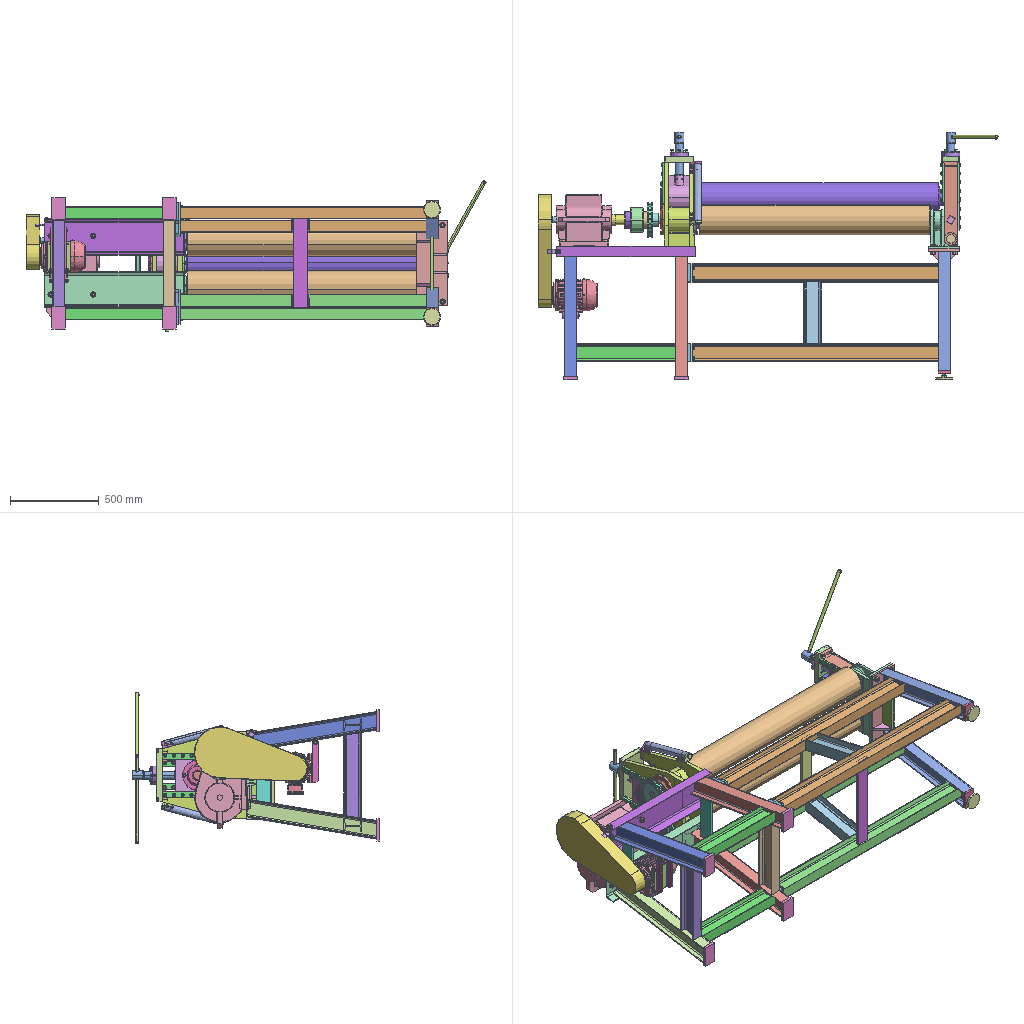Assembly | SolidWorks | 110 different items | 393 placed | box 2588 x 1390 x 851 mm
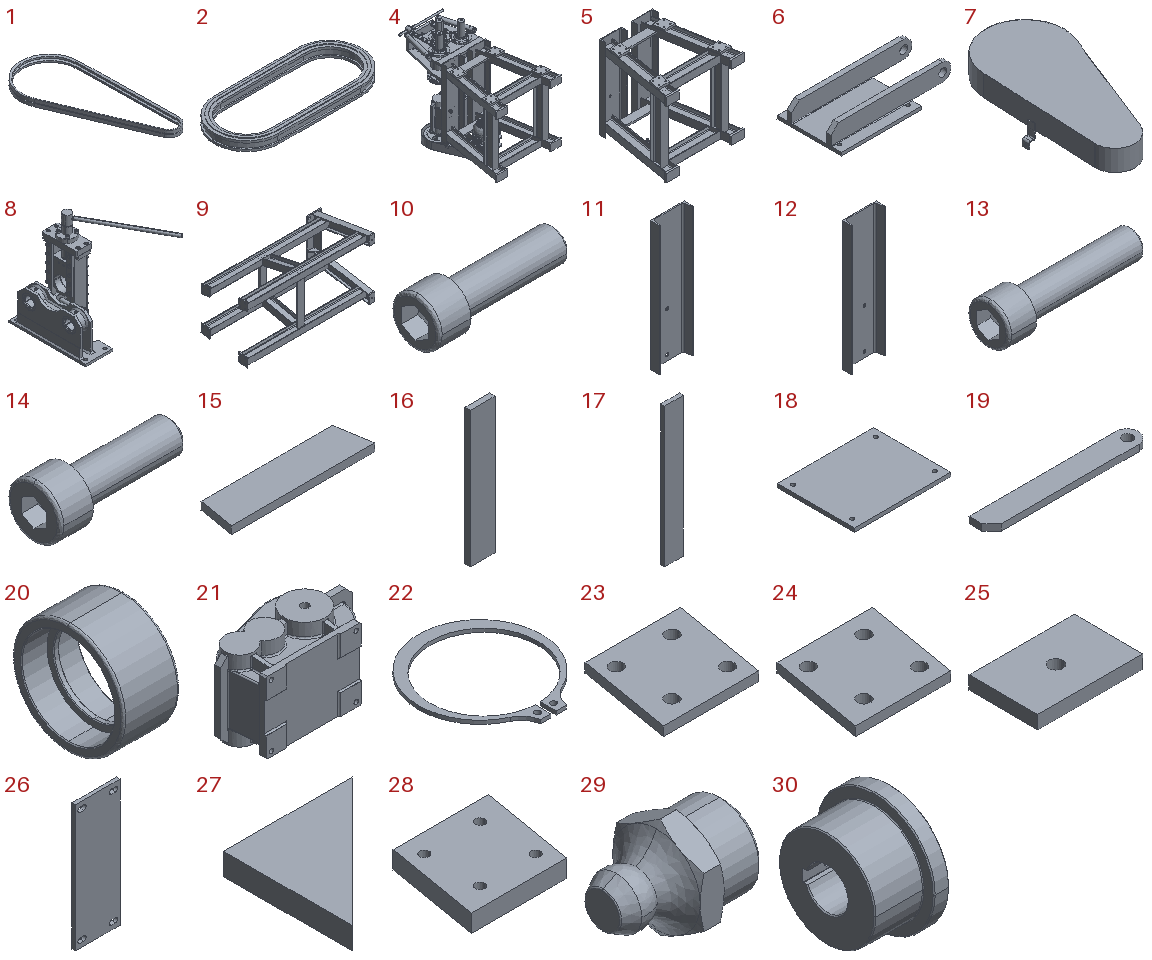Parts list (item | name | quantity | parent item | size | volume | features):
1 | (subassembly) | x1 | in 4 | 255.391 x 589.134 x 28.445 mm | 211928 mm3 | -
2 | (subassembly) | x1 | in 4 | 444.526 x 194.526 x 33.528 mm | 618540 mm3 | -
3 | (subassembly) | x1 | - | - | - | -
4 | (subassembly) | x1 | - | - | 68898357 mm3 | -
5 | (subassembly) | x1 | in 4 | 738.903 x 747.997 x 780 mm | 12463508 mm3 | -
6 | (subassembly) | x1 | in 4 | 244.844 x 131 x 41.4 mm | 299853 mm3 | -
7 | (subassembly) | x1 | in 4 | 319.788 x 636.5 x 127.78 mm | 416988 mm3 | -
8 | (subassembly) | x1 | - | 388.966 x 706.727 x 655.972 mm | 9412553 mm3 | -
9 | (subassembly) | x1 | - | 1510 x 699 x 705.243 mm | 14014214 mm3 | -
10 | - | x4 | in 8 | 52 x 18 x 18 mm | 6907 mm3 | features BaseBody 1
11 | - | x1 | in 5 | 203.2 x 57.4 x 780 mm | 1609191 mm3 | features BaseBody 1
12 | - | x1 | in 5 | 203.2 x 57.4 x 780 mm | 1609191 mm3 | features BaseBody 1
13 | - | x12 | in 4, 8 | 62 x 18 x 18 mm | 8038 mm3 | features BaseBody 1
14 | - | x8 | in 4 | 33 x 13 x 13 mm | 2157 mm3 | features BaseBody 1
15 | - | x1 | in 9 | 300.429 x 76.2 x 16 mm | 350736 mm3 | features BaseBody 1
16 | - | x1 | in 9 | 76 x 16 x 413.5 mm | 502816 mm3 | features BaseBody 1
17 | - | x1 | in 9 | 76 x 16 x 563.5 mm | 685216 mm3 | features BaseBody 1
18 | - | x1 | in 6 | 164 x 131 x 6.4 mm | 136609 mm3 | features BaseBody 1
19 | - | x2 | in 6 | 244.844 x 35 x 10 mm | 81253 mm3 | features BaseBody 1
20 | - | x1 | in 4 | 70 x 138 x 138 mm | 337126 mm3 | features BaseBody 1
21 | - | x1 | in 4 | 510 x 292.394 x 310 mm | 26978776 mm3 | features BaseBody 1
22 | - | x3 | in 4 | 54 x 59.172 x 1.6 mm | 946.092 mm3 | features BaseBody 1
23 | - | x2 | in 9 | 120.015 x 101.6 x 10 mm | 98503 mm3 | features BaseBody 1
24 | - | x2 | in 9 | 120.015 x 101.6 x 10 mm | 98503 mm3 | features BaseBody 1
25 | - | x2 | in 9 | 103 x 67.6 x 13 mm | 88562 mm3 | features BaseBody 1
26 | - | x1 | in 9 | 170 x 13 x 480 mm | 1034464 mm3 | features BaseBody 1
27 | - | x4 | in 9 | 76 x 76 x 13 mm | 37544 mm3 | features BaseBody 1
28 | - | x4 | in 5 | 120.015 x 101.6 x 19 mm | 192760 mm3 | features BaseBody 1
29 | - | x3 | in 8 | 16 x 11 x 12.702 mm | 986.989 mm3 | features BaseBody 1
30 | - | x1 | in 4 | 65 x 115 x 115 mm | 415156 mm3 | features BaseBody 1
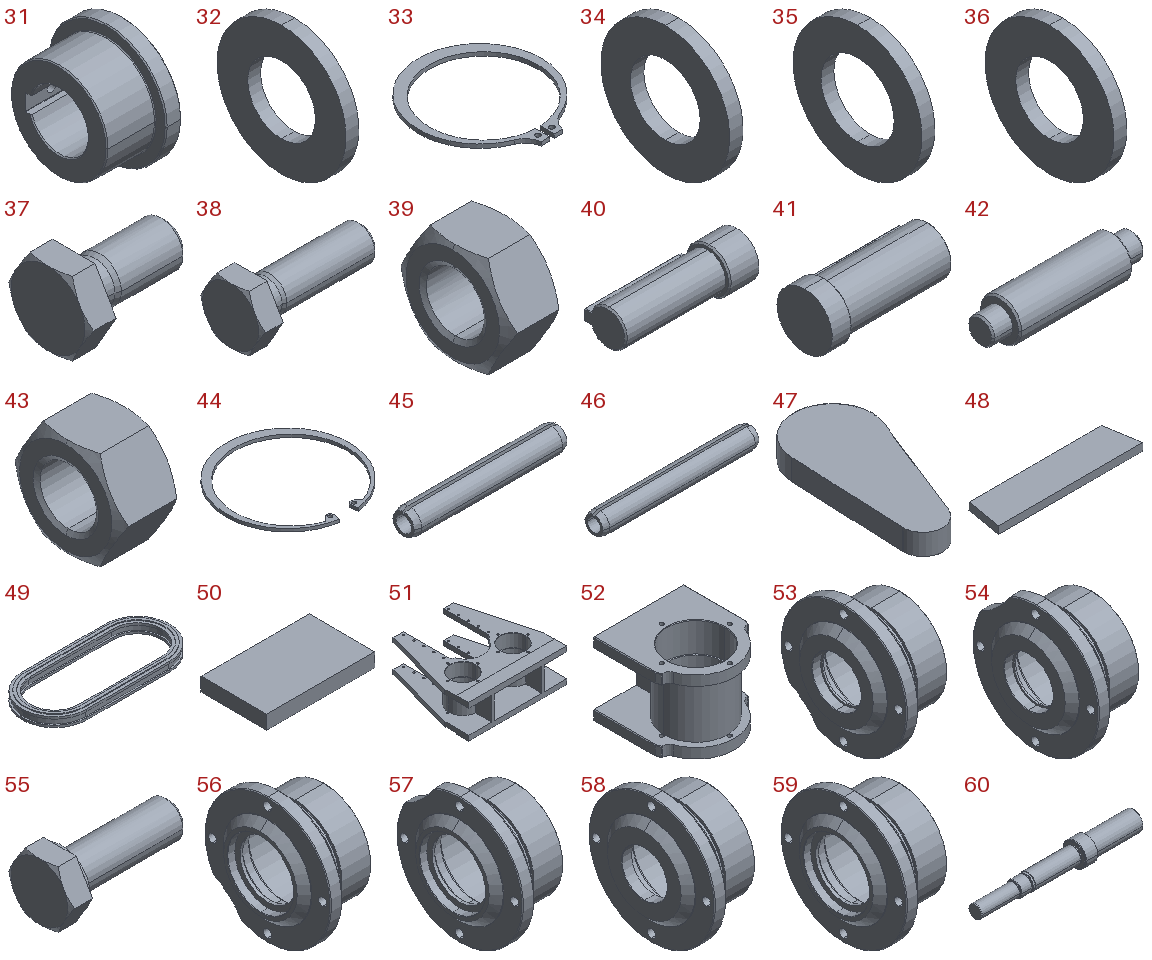31 | - | x1 | in 4 | 65 x 115 x 115 mm | 335130 mm3 | features BaseBody 1
32 | - | x70 | in 4, 8 | 2 x 20 x 20 mm | 455.138 mm3 | features BaseBody 1
33 | - | x1 | - | 64.433 x 69.873 x 2 mm | 1579 mm3 | features BaseBody 1
34 | - | x16 | - | 2.5 x 24 x 24 mm | 799.143 mm3 | features BaseBody 1
35 | - | x16 | in 4 | 3 x 30 x 30 mm | 1440 mm3 | features BaseBody 1
36 | - | x4 | in 4 | 1.6 x 16 x 16 mm | 233.031 mm3 | features BaseBody 1
37 | - | x2 | in 4 | 16 x 11.547 x 10 mm | 654.588 mm3 | features BaseBody 1
38 | - | x4 | in 4 | 30.3 x 15.011 x 13 mm | 1969 mm3 | features BaseBody 1
39 | - | x4 | in 4 | 13 x 27.713 x 24 mm | 4387 mm3 | features BaseBody 1
40 | - | x1 | in 4 | 93 x 33 x 32 mm | 57387 mm3 | features BaseBody 1
41 | - | x1 | in 4 | 145 x 66.5 x 65 mm | 388822 mm3 | features BaseBody 1
42 | - | x1 | in 5 | 94 x 25.4 x 25.4 mm | 40077 mm3 | features BaseBody 1
43 | - | x4 | - | 14.8 x 27.713 x 24 mm | 5033 mm3 | features BaseBody 1
44 | - | x6 | in 4 | 116.7 x 115.986 x 2.8 mm | 5057 mm3 | features BaseBody 1
45 | - | x2 | in 4 | 50 x 8 x 7.968 mm | 1446 mm3 | features BaseBody 1
46 | - | x2 | in 8 | 60 x 8 x 7.968 mm | 1740 mm3 | features BaseBody 1
47 | - | x1 | in 7 | 306.5 x 636.5 x 76.6 mm | 401718 mm3 | features BaseBody 1
48 | - | x2 | in 5 | 310.603 x 76.2 x 16 mm | 363141 mm3 | features BaseBody 1
49 | - | x1 | in 2 | 444.526 x 194.526 x 33.528 mm | 618540 mm3 | features BaseBody 1
50 | - | x4 | in 5 | 125 x 76.2 x 16 mm | 152400 mm3 | features BaseBody 1
51 | - | x1 | in 4 | 490 x 474 x 167.3 mm | 6268436 mm3 | features BaseBody 1
52 | - | x1 | in 4 | 200 x 210 x 160.5 mm | 1529038 mm3 | features BaseBody 1
53 | - | x1 | in 4 | 86.84 x 172 x 172 mm | 547122 mm3 | features BaseBody 1
54 | - | x1 | in 4 | 86.84 x 172 x 172 mm | 547344 mm3 | features BaseBody 1
55 | - | x26 | in 8 | 36.4 x 18.475 x 16 mm | 3746 mm3 | features BaseBody 1
56 | - | x1 | in 4 | 86.84 x 172 x 172 mm | 513296 mm3 | features BaseBody 1
57 | - | x1 | in 4 | 86.84 x 172 x 172 mm | 513518 mm3 | features BaseBody 1
58 | - | x1 | in 4 | 86.84 x 172 x 172 mm | 557963 mm3 | features BaseBody 1
59 | - | x1 | in 4 | 86.84 x 172 x 172 mm | 518697 mm3 | features BaseBody 1
60 | - | x1 | in 4 | 498.34 x 74 x 74 mm | 1078927 mm3 | features BaseBody 1
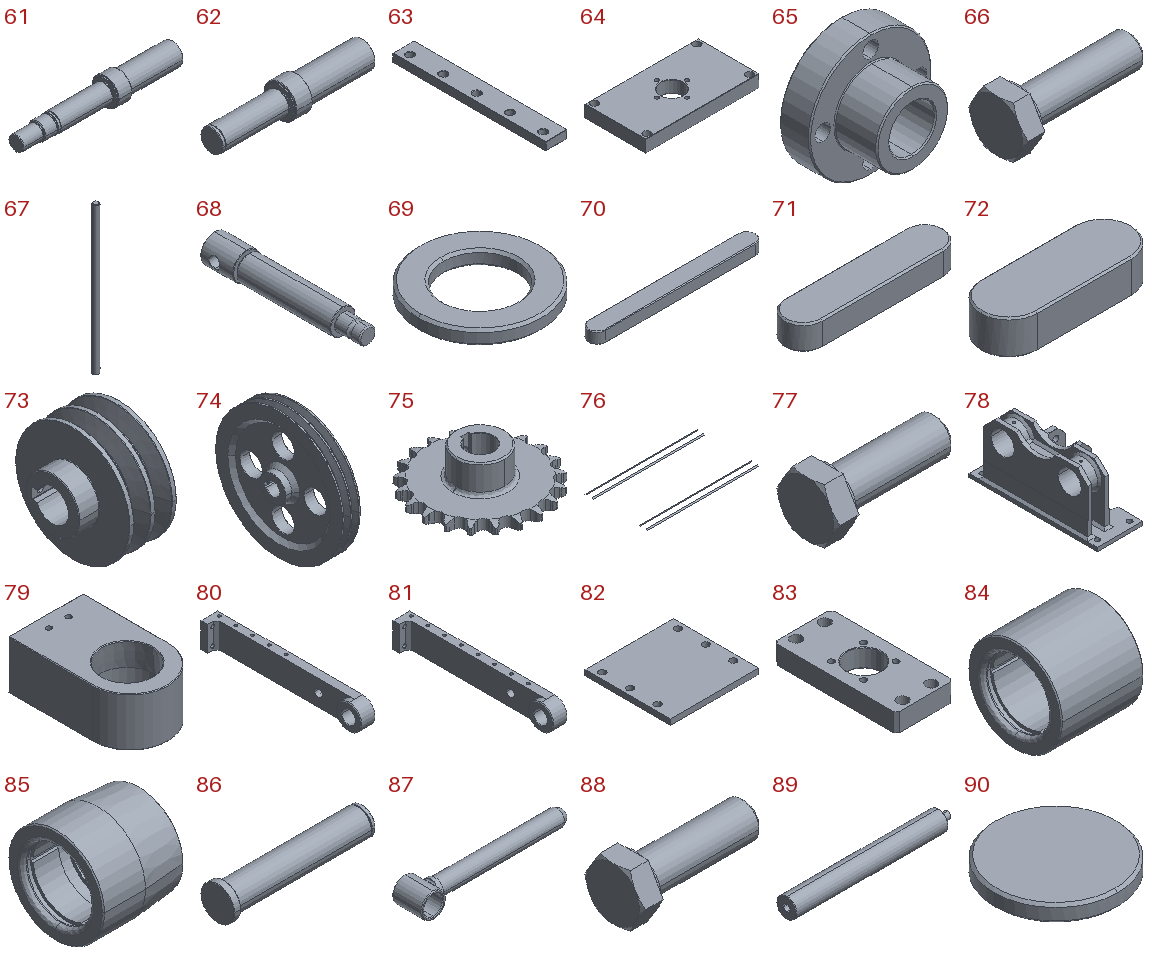61 | - | x1 | in 4 | 434.34 x 74 x 74 mm | 1002154 mm3 | features BaseBody 1
62 | - | x1 | in 4 | 341.34 x 74 x 74 mm | 870212 mm3 | features BaseBody 1
63 | - | x8 | in 4, 8 | 32 x 230 x 12 mm | 82466 mm3 | features BaseBody 1
64 | - | x1 | in 4 | 300 x 160.5 x 32 mm | 1414203 mm3 | features BaseBody 1
65 | - | x2 | in 4, 8 | 102 x 60 x 102 mm | 221417 mm3 | features BaseBody 1
66 | - | x44 | in 4 | 41.4 x 18.475 x 16 mm | 4138 mm3 | features BaseBody 1
67 | - | x2 | in 4, 8 | 23.05 x 19.05 x 500 mm | 142580 mm3 | features BaseBody 1
68 | - | x2 | in 4, 8 | 50.8 x 282 x 50.8 mm | 426019 mm3 | features BaseBody 1
69 | - | x2 | in 4, 8 | 50.8 x 50.8 x 6 mm | 7609 mm3 | features BaseBody 1
70 | - | x1 | in 4 | 116 x 12 x 8 mm | 10828 mm3 | features BaseBody 1
71 | - | x1 | in 4 | 51 x 12 x 8 mm | 4620 mm3 | features BaseBody 1
72 | - | x3 | in 4 | 48 x 18 x 11 mm | 8710 mm3 | features BaseBody 1
73 | - | x1 | in 4 | 50 x 85 x 85 mm | 143895 mm3 | features BaseBody 1
74 | - | x1 | in 4 | 47.331 x 248 x 248 mm | 1015220 mm3 | features BaseBody 1
75 | - | x2 | in 4 | 183.758 x 182.894 x 56.916 mm | 418597 mm3 | features BaseBody 1
76 | - | x1 | in 6 | 164 x 93 x 1.5 mm | 738 mm3 | features BaseBody 4
77 | - | x16 | - | 42.5 x 20.785 x 18 mm | 6020 mm3 | features BaseBody 1
78 | - | x1 | in 8 | 170 x 480 x 224 mm | 3738695 mm3 | features BaseBody 1
79 | - | x1 | in 8 | 115 x 187.5 x 75 mm | 1043413 mm3 | features BaseBody 1
80 | - | x1 | in 8 | 50 x 470 x 75 mm | 866067 mm3 | features BaseBody 1
81 | - | x1 | in 8 | 50 x 470 x 75 mm | 866067 mm3 | features BaseBody 1
82 | - | x1 | in 8 | 160 x 155 x 10 mm | 241214 mm3 | features BaseBody 1
83 | - | x1 | in 8 | 100 x 215 x 32 mm | 560281 mm3 | features BaseBody 1
84 | - | x2 | in 8 | 76 x 86 x 86 mm | 218570 mm3 | features BaseBody 1
85 | - | x1 | - | 75 x 85 x 85 mm | 185357 mm3 | features BaseBody 1
86 | - | x1 | in 8 | 215 x 50 x 50 mm | 276823 mm3 | features BaseBody 1
87 | - | x1 | in 8 | 211.2 x 40 x 33.4 mm | 81310 mm3 | features BaseBody 1
88 | - | x10 | in 4 | 60 x 27.713 x 24 mm | 14953 mm3 | features BaseBody 1
89 | - | x2 | - | 1379 x 168 x 168 mm | 11660432 mm3 | features BaseBody 1
90 | - | x2 | - | 95 x 95 x 13 mm | 90970 mm3 | features BaseBody 1
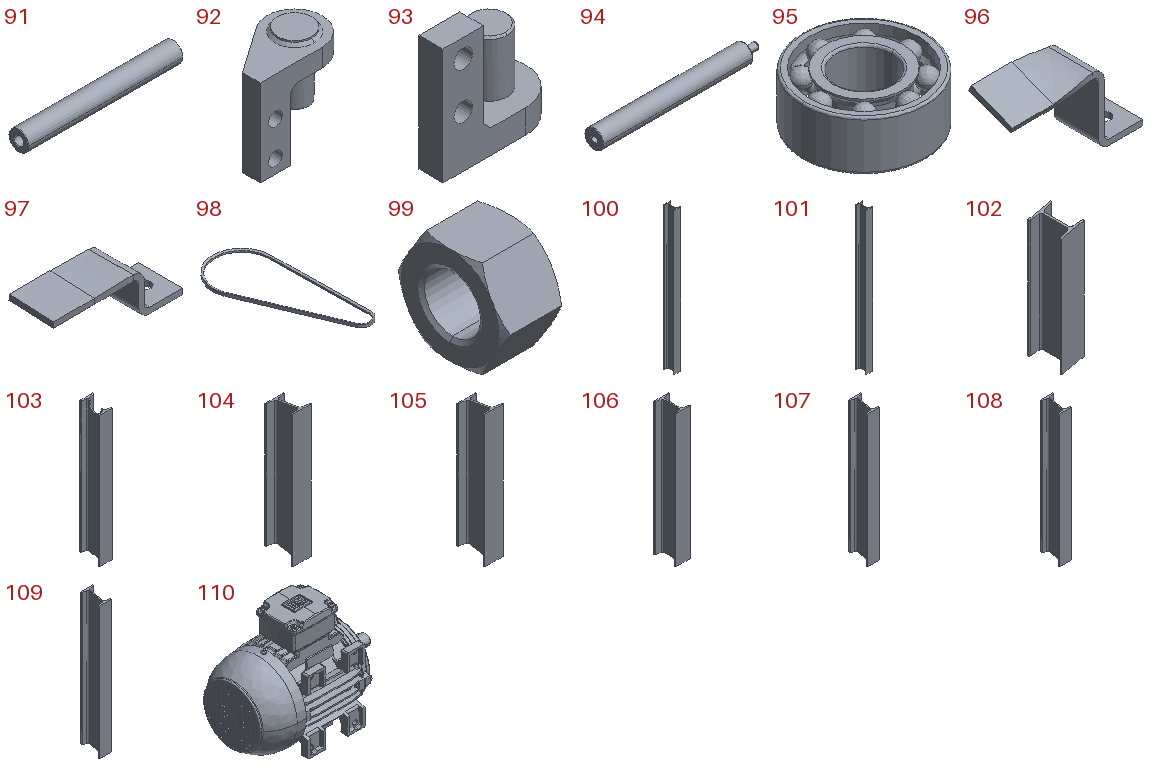91 | - | x2 | in 4 | 330 x 42.2 x 42.2 mm | 188080 mm3 | features BaseBody 1
92 | - | x2 | in 4 | 65 x 40 x 66 mm | 48299 mm3 | features BaseBody 1
93 | - | x2 | in 4 | 65 x 40 x 66 mm | 48299 mm3 | features BaseBody 1
94 | - | x1 | - | 1461 x 168 x 168 mm | 11688536 mm3 | features BaseBody 1
95 | - | x6 | in 4 | - | - | features RefSurface 16, BaseBody 2
96 | - | x1 | in 7 | 73.18 x 25.199 x 44.598 mm | 8281 mm3 | features BaseBody 1
97 | - | x1 | in 7 | 73.18 x 25.116 x 24.356 mm | 6989 mm3 | features BaseBody 1
98 | - | x2 | in 1 | 255.391 x 589.134 x 12.57 mm | 105964 mm3 | features BaseBody 1
99 | - | x2 | - | 14.8 x 27.713 x 24 mm | 5097 mm3 | features BaseBody 1
100 | - | x2 | in 9 | 67.6 x 101.6 x 1413 mm | 1963956 mm3 | features BaseBody 1
101 | - | x2 | in 9 | 67.6 x 101.6 x 1413 mm | 1963956 mm3 | features BaseBody 1
102 | - | x2 | in 9 | 67.6 x 101.6 x 369.5 mm | 493243 mm3 | features BaseBody 1
103 | - | x2 | in 9 | 67.6 x 101.6 x 699.36 mm | 938679 mm3 | features BaseBody 1
104 | - | x1 | in 5 | 67.6 x 101.6 x 482.765 mm | 647373 mm3 | features BaseBody 1
105 | - | x1 | in 5 | 67.6 x 101.6 x 482.765 mm | 647373 mm3 | features BaseBody 1
106 | - | x2 | in 5 | 67.6 x 101.6 x 617.6 mm | 858414 mm3 | features BaseBody 1
107 | - | x2 | in 5 | 67.6 x 101.6 x 753.5 mm | 1021639 mm3 | features BaseBody 1
108 | - | x1 | in 5 | 67.6 x 101.6 x 753.5 mm | 1021639 mm3 | features BaseBody 1
109 | - | x1 | in 5 | 67.6 x 101.6 x 753.5 mm | 1021639 mm3 | features BaseBody 1
110 | - | x1 | in 4 | 304.5 x 182.47 x 241.47 mm | 5604300 mm3 | features BaseBody 1